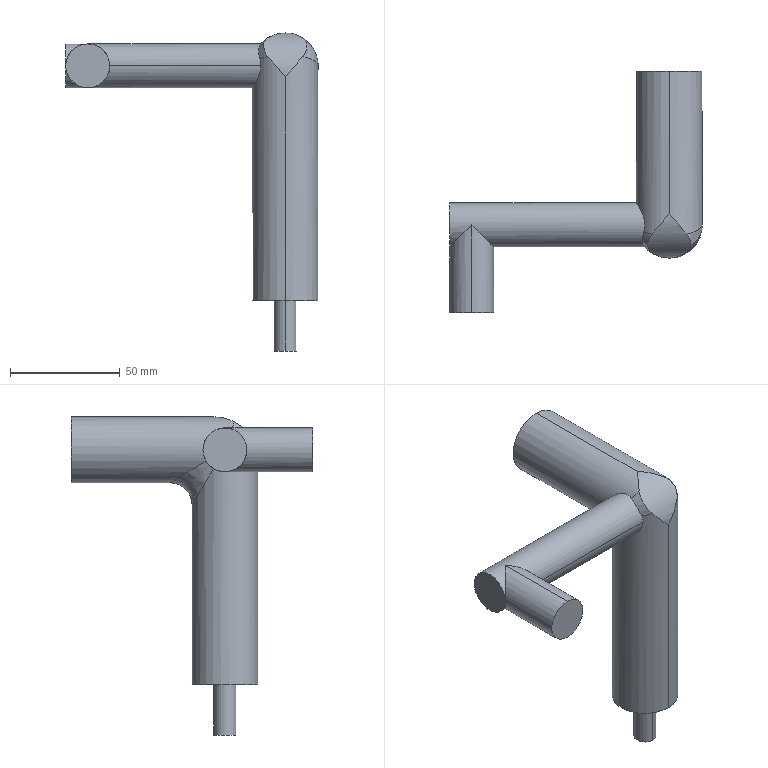Part | SolidWorks | features BaseBody 1 | 1 solid | 19 faces | box 115 x 110 x 145 mm | volume 163040 mm3 | cylinder 11 | plane 5 | spline 3 | commonest cylinder face diameters 20 x4 30 x4 10 x2 40 x1
STEP:
#1=CARTESIAN_POINT('',(268.959,17.138,-340.));
#2=VERTEX_POINT('',#1);
#3=CARTESIAN_POINT('',(268.959,17.138,-360.));
#4=VERTEX_POINT('',#3);
#5=CARTESIAN_POINT('',(268.959,17.138,-350.));
#6=DIRECTION('',(0.,-1.,0.));
#7=DIRECTION('',(0.,0.,1.));
#8=AXIS2_PLACEMENT_3D('',#5,#6,#7);
#9=CIRCLE('',#8,10.);
#10=EDGE_CURVE('',#2,#4,#9,.T.);
#11=ORIENTED_EDGE('',*,*,#10,.F.);
#12=CARTESIAN_POINT('',(268.959,57.138,-340.));
#13=VERTEX_POINT('',#12);
#14=CARTESIAN_POINT('',(268.959,17.138,-340.));
#15=DIRECTION('',(0.,1.,0.));
#16=VECTOR('',#15,1000.);
#17=LINE('',#14,#16);
#18=EDGE_CURVE('',#2,#13,#17,.T.);
#19=ORIENTED_EDGE('',*,*,#18,.T.);
#20=CARTESIAN_POINT('',(258.959,47.138,-350.));
#21=VERTEX_POINT('',#20);
#22=CARTESIAN_POINT('',(268.959,57.138,-340.));
#23=CARTESIAN_POINT('',(263.101,51.28,-340.));
#24=CARTESIAN_POINT('',(258.959,47.138,-344.142));
#25=CARTESIAN_POINT('',(258.959,47.138,-350.));
#26=(BOUNDED_CURVE()B_SPLINE_CURVE(3,(#22,#23,#24,#25),.UNSPECIFIED.,.F.,.T.)B_SPLINE_CURVE_WITH_KNOTS((4,4),(1.571,3.142),.UNSPECIFIED.)CURVE()GEOMETRIC_REPRESENTATION_ITEM()RATIONAL_B_SPLINE_CURVE((1.,0.8047,0.8047,1.))REPRESENTATION_ITEM(''));
#27=EDGE_CURVE('',#13,#21,#26,.T.);
#28=ORIENTED_EDGE('',*,*,#27,.T.);
#29=CARTESIAN_POINT('',(268.959,57.138,-360.));
#30=VERTEX_POINT('',#29);
#31=CARTESIAN_POINT('',(258.959,47.138,-350.));
#32=CARTESIAN_POINT('',(258.959,47.138,-355.858));
#33=CARTESIAN_POINT('',(263.101,51.28,-360.));
#34=CARTESIAN_POINT('',(268.959,57.138,-360.));
#35=(BOUNDED_CURVE()B_SPLINE_CURVE(3,(#31,#32,#33,#34),.UNSPECIFIED.,.F.,.F.)B_SPLINE_CURVE_WITH_KNOTS((4,4),(3.142,4.712),.UNSPECIFIED.)CURVE()GEOMETRIC_REPRESENTATION_ITEM()RATIONAL_B_SPLINE_CURVE((1.,0.8047,0.8047,1.))REPRESENTATION_ITEM(''));
#36=EDGE_CURVE('',#21,#30,#35,.T.);
#37=ORIENTED_EDGE('',*,*,#36,.T.);
#38=CARTESIAN_POINT('',(268.959,17.138,-360.));
#39=DIRECTION('',(0.,1.,0.));
#40=VECTOR('',#39,1000.);
#41=LINE('',#38,#40);
#42=EDGE_CURVE('',#4,#30,#41,.T.);
#43=ORIENTED_EDGE('',*,*,#42,.F.);
#44=EDGE_LOOP('',(#11,#19,#28,#37,#43));
#45=FACE_OUTER_BOUND('',#44,.T.);
#46=CARTESIAN_POINT('',(268.959,17.138,-350.));
#47=DIRECTION('',(0.,1.,0.));
#48=DIRECTION('',(0.,0.,-1.));
#49=AXIS2_PLACEMENT_3D('',#46,#47,#48);
#50=CYLINDRICAL_SURFACE('',#49,10.);
#51=ADVANCED_FACE('',(#45),#50,.T.);
#52=CARTESIAN_POINT('',(358.959,52.138,-480.));
#53=VERTEX_POINT('',#52);
#54=CARTESIAN_POINT('',(358.959,62.138,-480.));
#55=VERTEX_POINT('',#54);
#56=CARTESIAN_POINT('',(358.959,57.138,-480.));
#57=DIRECTION('',(0.,0.,-1.));
#58=DIRECTION('',(0.,-1.,0.));
#59=AXIS2_PLACEMENT_3D('',#56,#57,#58);
#60=CIRCLE('',#59,5.);
#61=EDGE_CURVE('',#53,#55,#60,.T.);
#62=ORIENTED_EDGE('',*,*,#61,.F.);
#63=CARTESIAN_POINT('',(358.959,52.138,-457.));
#64=VERTEX_POINT('',#63);
#65=CARTESIAN_POINT('',(358.959,52.138,-480.));
#66=DIRECTION('',(0.,0.,1.));
#67=VECTOR('',#66,1000.);
#68=LINE('',#65,#67);
#69=EDGE_CURVE('',#53,#64,#68,.T.);
#70=ORIENTED_EDGE('',*,*,#69,.T.);
#71=CARTESIAN_POINT('',(358.959,62.138,-457.));
#72=VERTEX_POINT('',#71);
#73=CARTESIAN_POINT('',(358.959,57.138,-457.));
#74=DIRECTION('',(0.,0.,-1.));
#75=DIRECTION('',(0.,1.,0.));
#76=AXIS2_PLACEMENT_3D('',#73,#74,#75);
#77=CIRCLE('',#76,5.);
#78=EDGE_CURVE('',#64,#72,#77,.T.);
#79=ORIENTED_EDGE('',*,*,#78,.T.);
#80=CARTESIAN_POINT('',(358.959,62.138,-480.));
#81=DIRECTION('',(0.,0.,1.));
#82=VECTOR('',#81,1000.);
#83=LINE('',#80,#82);
#84=EDGE_CURVE('',#55,#72,#83,.T.);
#85=ORIENTED_EDGE('',*,*,#84,.F.);
#86=EDGE_LOOP('',(#62,#70,#79,#85));
#87=FACE_OUTER_BOUND('',#86,.T.);
#88=CARTESIAN_POINT('',(358.959,57.138,-480.));
#89=DIRECTION('',(0.,0.,1.));
#90=DIRECTION('',(0.,1.,0.));
#91=AXIS2_PLACEMENT_3D('',#88,#89,#90);
#92=CYLINDRICAL_SURFACE('',#91,5.);
#93=ADVANCED_FACE('',(#87),#92,.T.);
#94=CARTESIAN_POINT('',(344.869,62.283,-358.575));
#95=VERTEX_POINT('',#94);
#96=CARTESIAN_POINT('',(358.959,72.138,-375.));
#97=VERTEX_POINT('',#96);
#98=CARTESIAN_POINT('',(344.869,62.283,-358.575));
#99=CARTESIAN_POINT('',(347.104,68.404,-368.776));
#100=CARTESIAN_POINT('',(352.443,72.138,-375.));
#101=CARTESIAN_POINT('',(358.959,72.138,-375.));
#102=(BOUNDED_CURVE()B_SPLINE_CURVE(3,(#98,#99,#100,#101),.UNSPECIFIED.,.F.,.T.)B_SPLINE_CURVE_WITH_KNOTS((4,4),(5.062,6.283),.UNSPECIFIED.)CURVE()GEOMETRIC_REPRESENTATION_ITEM()RATIONAL_B_SPLINE_CURVE((1.,0.8796,0.8796,1.))REPRESENTATION_ITEM(''));
#103=EDGE_CURVE('',#95,#97,#102,.T.);
#104=ORIENTED_EDGE('',*,*,#103,.T.);
#105=CARTESIAN_POINT('',(358.959,72.138,-457.));
#106=VERTEX_POINT('',#105);
#107=CARTESIAN_POINT('',(358.959,72.138,-307.574));
#108=DIRECTION('',(0.,0.,-1.));
#109=VECTOR('',#108,1000.);
#110=LINE('',#107,#109);
#111=EDGE_CURVE('',#97,#106,#110,.T.);
#112=ORIENTED_EDGE('',*,*,#111,.T.);
#113=CARTESIAN_POINT('',(358.959,42.138,-457.));
#114=VERTEX_POINT('',#113);
#115=CARTESIAN_POINT('',(358.959,57.138,-457.));
#116=DIRECTION('',(0.,0.,1.));
#117=DIRECTION('',(0.,1.,0.));
#118=AXIS2_PLACEMENT_3D('',#115,#116,#117);
#119=CIRCLE('',#118,15.);
#120=EDGE_CURVE('',#106,#114,#119,.T.);
#121=ORIENTED_EDGE('',*,*,#120,.T.);
#122=CARTESIAN_POINT('',(358.959,42.138,-355.));
#123=VERTEX_POINT('',#122);
#124=CARTESIAN_POINT('',(358.959,42.138,-307.574));
#125=DIRECTION('',(0.,0.,-1.));
#126=VECTOR('',#125,1000.);
#127=LINE('',#124,#126);
#128=EDGE_CURVE('',#123,#114,#127,.T.);
#129=ORIENTED_EDGE('',*,*,#128,.F.);
#130=CARTESIAN_POINT('',(351.033,44.403,-345.755));
#131=VERTEX_POINT('',#130);
#132=CARTESIAN_POINT('',(358.959,42.138,-355.));
#133=CARTESIAN_POINT('',(358.789,42.138,-354.804));
#134=CARTESIAN_POINT('',(358.618,42.141,-354.606));
#135=CARTESIAN_POINT('',(358.277,42.153,-354.212));
#136=CARTESIAN_POINT('',(358.106,42.162,-354.015));
#137=CARTESIAN_POINT('',(357.596,42.197,-353.426));
#138=CARTESIAN_POINT('',(357.257,42.231,-353.034));
#139=CARTESIAN_POINT('',(356.242,42.371,-351.86));
#140=CARTESIAN_POINT('',(355.569,42.51,-351.08));
#141=CARTESIAN_POINT('',(354.567,42.792,-349.915));
#142=CARTESIAN_POINT('',(354.234,42.898,-349.526));
#143=CARTESIAN_POINT('',(353.574,43.134,-348.756));
#144=CARTESIAN_POINT('',(353.248,43.264,-348.374));
#145=CARTESIAN_POINT('',(352.28,43.689,-347.236));
#146=CARTESIAN_POINT('',(351.649,44.02,-346.49));
#147=CARTESIAN_POINT('',(351.033,44.403,-345.755));
#148=B_SPLINE_CURVE_WITH_KNOTS('',3,(#132,#133,#134,#135,#136,#137,#138,#139,#140,#141,#142,#143,#144,#145,#146,#147),.UNSPECIFIED.,.F.,.F.,(4,2,2,2,2,2,2,4),(-0.00002828,0.0007507,0.00153,0.003088,0.006204,0.007762,0.00932,0.01244),.UNSPECIFIED.);
#149=EDGE_CURVE('',#123,#131,#148,.T.);
#150=ORIENTED_EDGE('',*,*,#149,.T.);
#151=CARTESIAN_POINT('',(347.34,47.652,-346.838));
#152=VERTEX_POINT('',#151);
#153=CARTESIAN_POINT('',(351.033,44.403,-345.755));
#154=CARTESIAN_POINT('',(349.629,45.277,-346.046));
#155=CARTESIAN_POINT('',(348.386,46.37,-346.411));
#156=CARTESIAN_POINT('',(347.34,47.652,-346.838));
#157=(BOUNDED_CURVE()B_SPLINE_CURVE(3,(#153,#154,#155,#156),.UNSPECIFIED.,.F.,.F.)B_SPLINE_CURVE_WITH_KNOTS((4,4),(3.698,4.028),.UNSPECIFIED.)CURVE()GEOMETRIC_REPRESENTATION_ITEM()RATIONAL_B_SPLINE_CURVE((1.,0.991,0.991,1.))REPRESENTATION_ITEM(''));
#158=EDGE_CURVE('',#131,#152,#157,.T.);
#159=ORIENTED_EDGE('',*,*,#158,.T.);
#160=CARTESIAN_POINT('',(347.779,47.138,-350.));
#161=VERTEX_POINT('',#160);
#162=CARTESIAN_POINT('',(347.779,47.138,-350.));
#163=CARTESIAN_POINT('',(347.779,47.138,-349.458));
#164=CARTESIAN_POINT('',(347.739,47.182,-348.921));
#165=CARTESIAN_POINT('',(347.626,47.312,-348.125));
#166=CARTESIAN_POINT('',(347.579,47.367,-347.859));
#167=CARTESIAN_POINT('',(347.47,47.495,-347.341));
#168=CARTESIAN_POINT('',(347.408,47.569,-347.087));
#169=CARTESIAN_POINT('',(347.34,47.652,-346.838));
#170=B_SPLINE_CURVE_WITH_KNOTS('',3,(#162,#163,#164,#165,#166,#167,#168,#169),.UNSPECIFIED.,.F.,.F.,(4,2,2,4),(0.0323,0.03391,0.03472,0.03552),.UNSPECIFIED.);
#171=EDGE_CURVE('',#161,#152,#170,.T.);
#172=ORIENTED_EDGE('',*,*,#171,.F.);
#173=CARTESIAN_POINT('',(344.869,62.283,-358.575));
#174=CARTESIAN_POINT('',(344.735,61.916,-358.796));
#175=CARTESIAN_POINT('',(344.611,61.532,-358.994));
#176=CARTESIAN_POINT('',(344.445,60.931,-359.256));
#177=CARTESIAN_POINT('',(344.393,60.726,-359.337));
#178=CARTESIAN_POINT('',(344.296,60.307,-359.487));
#179=CARTESIAN_POINT('',(344.251,60.092,-359.556));
#180=CARTESIAN_POINT('',(344.052,59.017,-359.862));
#181=CARTESIAN_POINT('',(343.964,58.133,-359.992));
#182=CARTESIAN_POINT('',(343.958,56.994,-360.002));
#183=CARTESIAN_POINT('',(343.962,56.764,-359.996));
#184=CARTESIAN_POINT('',(343.98,56.31,-359.968));
#185=CARTESIAN_POINT('',(343.995,56.085,-359.947));
#186=CARTESIAN_POINT('',(344.052,55.414,-359.861));
#187=CARTESIAN_POINT('',(344.11,54.974,-359.773));
#188=CARTESIAN_POINT('',(344.262,54.108,-359.54));
#189=CARTESIAN_POINT('',(344.357,53.682,-359.394));
#190=CARTESIAN_POINT('',(344.573,52.87,-359.054));
#191=CARTESIAN_POINT('',(344.695,52.48,-358.859));
#192=CARTESIAN_POINT('',(344.963,51.729,-358.422));
#193=CARTESIAN_POINT('',(345.109,51.368,-358.178));
#194=CARTESIAN_POINT('',(345.411,50.69,-357.655));
#195=CARTESIAN_POINT('',(345.568,50.371,-357.375));
#196=CARTESIAN_POINT('',(345.888,49.772,-356.776));
#197=CARTESIAN_POINT('',(346.052,49.489,-356.455));
#198=CARTESIAN_POINT('',(346.376,48.968,-355.781));
#199=CARTESIAN_POINT('',(346.534,48.73,-355.43));
#200=CARTESIAN_POINT('',(346.837,48.3,-354.698));
#201=CARTESIAN_POINT('',(346.98,48.108,-354.317));
#202=CARTESIAN_POINT('',(347.244,47.768,-353.519));
#203=CARTESIAN_POINT('',(347.365,47.62,-353.1));
#204=CARTESIAN_POINT('',(347.563,47.383,-352.244));
#205=CARTESIAN_POINT('',(347.642,47.293,-351.808));
#206=CARTESIAN_POINT('',(347.75,47.17,-350.915));
#207=CARTESIAN_POINT('',(347.779,47.138,-350.454));
#208=CARTESIAN_POINT('',(347.779,47.138,-350.));
#209=B_SPLINE_CURVE_WITH_KNOTS('',3,(#173,#174,#175,#176,#177,#178,#179,#180,#181,#182,#183,#184,#185,#186,#187,#188,#189,#190,#191,#192,#193,#194,#195,#196,#197,#198,#199,#200,#201,#202,#203,#204,#205,#206,#207,#208),.UNSPECIFIED.,.F.,.F.,(4,2,2,2,2,2,2,2,2,2,2,2,2,2,2,2,2,4),(0.01069,0.01204,0.01272,0.01339,0.01609,0.01677,0.01744,0.01879,0.02014,0.02149,0.02285,0.0242,0.02555,0.0269,0.02825,0.0296,0.03095,0.0323),.UNSPECIFIED.);
#210=EDGE_CURVE('',#95,#161,#209,.T.);
#211=ORIENTED_EDGE('',*,*,#210,.F.);
#212=EDGE_LOOP('',(#104,#112,#121,#129,#150,#159,#172,#211));
#213=FACE_OUTER_BOUND('',#212,.T.);
#214=CARTESIAN_POINT('',(358.959,57.138,-307.574));
#215=DIRECTION('',(0.,0.,-1.));
#216=DIRECTION('',(0.,-1.,0.));
#217=AXIS2_PLACEMENT_3D('',#214,#215,#216);
#218=CYLINDRICAL_SURFACE('',#217,15.);
#219=ADVANCED_FACE('',(#213),#218,.T.);
#220=CARTESIAN_POINT('',(358.959,62.138,-335.));
#221=VERTEX_POINT('',#220);
#222=CARTESIAN_POINT('',(351.033,52.893,-337.265));
#223=VERTEX_POINT('',#222);
#224=CARTESIAN_POINT('',(358.959,62.138,-335.));
#225=CARTESIAN_POINT('',(358.789,61.942,-335.));
#226=CARTESIAN_POINT('',(358.618,61.744,-335.003));
#227=CARTESIAN_POINT('',(358.277,61.35,-335.015));
#228=CARTESIAN_POINT('',(358.106,61.154,-335.023));
#229=CARTESIAN_POINT('',(357.596,60.564,-335.058));
#230=CARTESIAN_POINT('',(357.257,60.172,-335.093));
#231=CARTESIAN_POINT('',(356.242,58.998,-335.232));
#232=CARTESIAN_POINT('',(355.569,58.219,-335.372));
#233=CARTESIAN_POINT('',(354.567,57.053,-335.653));
#234=CARTESIAN_POINT('',(354.234,56.664,-335.76));
#235=CARTESIAN_POINT('',(353.574,55.894,-335.995));
#236=CARTESIAN_POINT('',(353.248,55.512,-336.125));
#237=CARTESIAN_POINT('',(352.28,54.375,-336.551));
#238=CARTESIAN_POINT('',(351.649,53.628,-336.882));
#239=CARTESIAN_POINT('',(351.033,52.893,-337.265));
#240=B_SPLINE_CURVE_WITH_KNOTS('',3,(#224,#225,#226,#227,#228,#229,#230,#231,#232,#233,#234,#235,#236,#237,#238,#239),.UNSPECIFIED.,.F.,.F.,(4,2,2,2,2,2,2,4),(-0.00002828,0.0007507,0.00153,0.003088,0.006204,0.007762,0.00932,0.01244),.UNSPECIFIED.);
#241=EDGE_CURVE('',#221,#223,#240,.T.);
#242=ORIENTED_EDGE('',*,*,#241,.F.);
#243=CARTESIAN_POINT('',(358.959,127.138,-335.));
#244=VERTEX_POINT('',#243);
#245=CARTESIAN_POINT('',(358.959,57.138,-335.));
#246=DIRECTION('',(0.,1.,0.));
#247=VECTOR('',#246,1000.);
#248=LINE('',#245,#247);
#249=EDGE_CURVE('',#221,#244,#248,.T.);
#250=ORIENTED_EDGE('',*,*,#249,.T.);
#251=CARTESIAN_POINT('',(358.959,127.138,-365.));
#252=VERTEX_POINT('',#251);
#253=CARTESIAN_POINT('',(358.959,127.138,-350.));
#254=DIRECTION('',(0.,-1.,0.));
#255=DIRECTION('',(0.,0.,-1.));
#256=AXIS2_PLACEMENT_3D('',#253,#254,#255);
#257=CIRCLE('',#256,15.);
#258=EDGE_CURVE('',#244,#252,#257,.T.);
#259=ORIENTED_EDGE('',*,*,#258,.T.);
#260=CARTESIAN_POINT('',(358.959,82.138,-365.));
#261=VERTEX_POINT('',#260);
#262=CARTESIAN_POINT('',(358.959,57.138,-365.));
#263=DIRECTION('',(0.,1.,0.));
#264=VECTOR('',#263,1000.);
#265=LINE('',#262,#264);
#266=EDGE_CURVE('',#261,#252,#265,.T.);
#267=ORIENTED_EDGE('',*,*,#266,.F.);
#268=CARTESIAN_POINT('',(344.869,65.713,-355.145));
#269=VERTEX_POINT('',#268);
#270=CARTESIAN_POINT('',(358.959,82.138,-365.));
#271=CARTESIAN_POINT('',(352.443,82.138,-365.));
#272=CARTESIAN_POINT('',(347.104,75.914,-361.265));
#273=CARTESIAN_POINT('',(344.869,65.713,-355.145));
#274=(BOUNDED_CURVE()B_SPLINE_CURVE(3,(#270,#271,#272,#273),.UNSPECIFIED.,.F.,.F.)B_SPLINE_CURVE_WITH_KNOTS((4,4),(0.,1.221),.UNSPECIFIED.)CURVE()GEOMETRIC_REPRESENTATION_ITEM()RATIONAL_B_SPLINE_CURVE((1.,0.8796,0.8796,1.))REPRESENTATION_ITEM(''));
#275=EDGE_CURVE('',#261,#269,#274,.T.);
#276=ORIENTED_EDGE('',*,*,#275,.T.);
#277=CARTESIAN_POINT('',(343.959,67.138,-350.));
#278=VERTEX_POINT('',#277);
#279=CARTESIAN_POINT('',(344.869,65.713,-355.145));
#280=CARTESIAN_POINT('',(344.733,65.937,-354.772));
#281=CARTESIAN_POINT('',(344.608,66.137,-354.383));
#282=CARTESIAN_POINT('',(344.44,66.401,-353.775));
#283=CARTESIAN_POINT('',(344.388,66.483,-353.567));
#284=CARTESIAN_POINT('',(344.291,66.634,-353.144));
#285=CARTESIAN_POINT('',(344.246,66.703,-352.926));
#286=CARTESIAN_POINT('',(344.125,66.888,-352.269));
#287=CARTESIAN_POINT('',(344.064,66.981,-351.824));
#288=CARTESIAN_POINT('',(343.981,67.106,-350.922));
#289=CARTESIAN_POINT('',(343.959,67.138,-350.463));
#290=CARTESIAN_POINT('',(343.959,67.138,-350.));
#291=B_SPLINE_CURVE_WITH_KNOTS('',3,(#279,#280,#281,#282,#283,#284,#285,#286,#287,#288,#289,#290),.UNSPECIFIED.,.F.,.F.,(4,2,2,2,2,4),(0.05913,0.06049,0.06118,0.06186,0.06323,0.0646),.UNSPECIFIED.);
#292=EDGE_CURVE('',#269,#278,#291,.T.);
#293=ORIENTED_EDGE('',*,*,#292,.T.);
#294=CARTESIAN_POINT('',(347.34,53.976,-340.513));
#295=VERTEX_POINT('',#294);
#296=CARTESIAN_POINT('',(343.959,67.138,-350.));
#297=CARTESIAN_POINT('',(343.959,67.138,-349.179));
#298=CARTESIAN_POINT('',(344.026,67.039,-348.379));
#299=CARTESIAN_POINT('',(344.216,66.749,-347.209));
#300=CARTESIAN_POINT('',(344.295,66.628,-346.822));
#301=CARTESIAN_POINT('',(344.475,66.347,-346.081));
#302=CARTESIAN_POINT('',(344.577,66.186,-345.723));
#303=CARTESIAN_POINT('',(344.801,65.826,-345.032));
#304=CARTESIAN_POINT('',(344.923,65.626,-344.697));
#305=CARTESIAN_POINT('',(345.183,65.189,-344.055));
#306=CARTESIAN_POINT('',(345.319,64.955,-343.751));
#307=CARTESIAN_POINT('',(345.598,64.457,-343.175));
#308=CARTESIAN_POINT('',(345.741,64.193,-342.903));
#309=CARTESIAN_POINT('',(346.031,63.634,-342.388));
#310=CARTESIAN_POINT('',(346.178,63.338,-342.144));
#311=CARTESIAN_POINT('',(346.608,62.414,-341.471));
#312=CARTESIAN_POINT('',(346.882,61.754,-341.095));
#313=CARTESIAN_POINT('',(347.235,60.683,-340.641));
#314=CARTESIAN_POINT('',(347.344,60.308,-340.507));
#315=CARTESIAN_POINT('',(347.529,59.544,-340.286));
#316=CARTESIAN_POINT('',(347.605,59.156,-340.197));
#317=CARTESIAN_POINT('',(347.719,58.363,-340.067));
#318=CARTESIAN_POINT('',(347.756,57.957,-340.025));
#319=CARTESIAN_POINT('',(347.786,57.138,-339.992));
#320=CARTESIAN_POINT('',(347.779,56.732,-340.));
#321=CARTESIAN_POINT('',(347.721,55.927,-340.065));
#322=CARTESIAN_POINT('',(347.67,55.528,-340.122));
#323=CARTESIAN_POINT('',(347.53,54.736,-340.284));
#324=CARTESIAN_POINT('',(347.442,54.35,-340.389));
#325=CARTESIAN_POINT('',(347.34,53.976,-340.513));
#326=B_SPLINE_CURVE_WITH_KNOTS('',3,(#296,#297,#298,#299,#300,#301,#302,#303,#304,#305,#306,#307,#308,#309,#310,#311,#312,#313,#314,#315,#316,#317,#318,#319,#320,#321,#322,#323,#324,#325),.UNSPECIFIED.,.F.,.F.,(4,2,2,2,2,2,2,2,2,2,2,2,2,2,4),(0.,0.002425,0.003638,0.00485,0.006063,0.007275,0.008488,0.009701,0.01213,0.01334,0.01455,0.01576,0.01698,0.01819,0.0194),.UNSPECIFIED.);
#327=EDGE_CURVE('',#278,#295,#326,.T.);
#328=ORIENTED_EDGE('',*,*,#327,.T.);
#329=CARTESIAN_POINT('',(347.34,53.976,-340.513));
#330=CARTESIAN_POINT('',(348.386,53.549,-339.232));
#331=CARTESIAN_POINT('',(349.629,53.185,-338.139));
#332=CARTESIAN_POINT('',(351.033,52.893,-337.265));
#333=(BOUNDED_CURVE()B_SPLINE_CURVE(3,(#329,#330,#331,#332),.UNSPECIFIED.,.F.,.T.)B_SPLINE_CURVE_WITH_KNOTS((4,4),(2.256,2.585),.UNSPECIFIED.)CURVE()GEOMETRIC_REPRESENTATION_ITEM()RATIONAL_B_SPLINE_CURVE((1.,0.991,0.991,1.))REPRESENTATION_ITEM(''));
#334=EDGE_CURVE('',#295,#223,#333,.T.);
#335=ORIENTED_EDGE('',*,*,#334,.T.);
#336=EDGE_LOOP('',(#242,#250,#259,#267,#276,#293,#328,#335));
#337=FACE_OUTER_BOUND('',#336,.T.);
#338=CARTESIAN_POINT('',(358.959,57.138,-350.));
#339=DIRECTION('',(0.,1.,0.));
#340=DIRECTION('',(0.,0.,-1.));
#341=AXIS2_PLACEMENT_3D('',#338,#339,#340);
#342=CYLINDRICAL_SURFACE('',#341,15.);
#343=ADVANCED_FACE('',(#337),#342,.T.);
#344=CARTESIAN_POINT('',(278.959,47.138,-350.));
#345=VERTEX_POINT('',#344);
#346=CARTESIAN_POINT('',(278.959,47.138,-350.));
#347=CARTESIAN_POINT('',(278.959,47.138,-344.142));
#348=CARTESIAN_POINT('',(274.817,51.28,-340.));
#349=CARTESIAN_POINT('',(268.959,57.138,-340.));
#350=(BOUNDED_CURVE()B_SPLINE_CURVE(3,(#346,#347,#348,#349),.UNSPECIFIED.,.F.,.T.)B_SPLINE_CURVE_WITH_KNOTS((4,4),(0.,1.571),.UNSPECIFIED.)CURVE()GEOMETRIC_REPRESENTATION_ITEM()RATIONAL_B_SPLINE_CURVE((1.,0.8047,0.8047,1.))REPRESENTATION_ITEM(''));
#351=EDGE_CURVE('',#345,#13,#350,.T.);
#352=ORIENTED_EDGE('',*,*,#351,.F.);
#353=CARTESIAN_POINT('',(258.959,47.138,-350.));
#354=DIRECTION('',(1.,0.,0.));
#355=VECTOR('',#354,1000.);
#356=LINE('',#353,#355);
#357=EDGE_CURVE('',#345,#161,#356,.T.);
#358=ORIENTED_EDGE('',*,*,#357,.T.);
#359=ORIENTED_EDGE('',*,*,#171,.T.);
#360=CARTESIAN_POINT('',(347.34,47.652,-346.838));
#361=CARTESIAN_POINT('',(347.143,47.893,-346.114));
#362=CARTESIAN_POINT('',(346.996,48.215,-345.421));
#363=CARTESIAN_POINT('',(346.845,48.823,-344.432));
#364=CARTESIAN_POINT('',(346.807,49.049,-344.109));
#365=CARTESIAN_POINT('',(346.756,49.532,-343.496));
#366=CARTESIAN_POINT('',(346.744,49.791,-343.206));
#367=CARTESIAN_POINT('',(346.743,50.34,-342.656));
#368=CARTESIAN_POINT('',(346.756,50.631,-342.397));
#369=CARTESIAN_POINT('',(346.806,51.246,-341.911));
#370=CARTESIAN_POINT('',(346.845,51.567,-341.687));
#371=CARTESIAN_POINT('',(346.945,52.225,-341.282));
#372=CARTESIAN_POINT('',(347.007,52.563,-341.1));
#373=CARTESIAN_POINT('',(347.155,53.257,-340.776));
#374=CARTESIAN_POINT('',(347.242,53.614,-340.634));
#375=CARTESIAN_POINT('',(347.34,53.976,-340.513));
#376=B_SPLINE_CURVE_WITH_KNOTS('',3,(#360,#361,#362,#363,#364,#365,#366,#367,#368,#369,#370,#371,#372,#373,#374,#375),.UNSPECIFIED.,.F.,.F.,(4,2,2,2,2,2,2,4),(0.,0.002332,0.003498,0.004664,0.00583,0.006996,0.008162,0.009328),.UNSPECIFIED.);
#377=EDGE_CURVE('',#152,#295,#376,.T.);
#378=ORIENTED_EDGE('',*,*,#377,.T.);
#379=ORIENTED_EDGE('',*,*,#327,.F.);
#380=CARTESIAN_POINT('',(258.959,67.138,-350.));
#381=VERTEX_POINT('',#380);
#382=CARTESIAN_POINT('',(258.959,67.138,-350.));
#383=DIRECTION('',(1.,0.,0.));
#384=VECTOR('',#383,1000.);
#385=LINE('',#382,#384);
#386=EDGE_CURVE('',#381,#278,#385,.T.);
#387=ORIENTED_EDGE('',*,*,#386,.F.);
#388=CARTESIAN_POINT('',(258.959,57.138,-350.));
#389=DIRECTION('',(-1.,0.,0.));
#390=DIRECTION('',(0.,-1.,0.));
#391=AXIS2_PLACEMENT_3D('',#388,#389,#390);
#392=CIRCLE('',#391,10.);
#393=EDGE_CURVE('',#21,#381,#392,.T.);
#394=ORIENTED_EDGE('',*,*,#393,.F.);
#395=ORIENTED_EDGE('',*,*,#27,.F.);
#396=EDGE_LOOP('',(#352,#358,#359,#378,#379,#387,#394,#395));
#397=FACE_OUTER_BOUND('',#396,.T.);
#398=CARTESIAN_POINT('',(258.959,57.138,-350.));
#399=DIRECTION('',(1.,0.,0.));
#400=DIRECTION('',(0.,1.,0.));
#401=AXIS2_PLACEMENT_3D('',#398,#399,#400);
#402=CYLINDRICAL_SURFACE('',#401,10.);
#403=ADVANCED_FACE('',(#397),#402,.T.);
#404=ORIENTED_EDGE('',*,*,#357,.F.);
#405=CARTESIAN_POINT('',(268.959,57.138,-360.));
#406=CARTESIAN_POINT('',(274.817,51.28,-360.));
#407=CARTESIAN_POINT('',(278.959,47.138,-355.858));
#408=CARTESIAN_POINT('',(278.959,47.138,-350.));
#409=(BOUNDED_CURVE()B_SPLINE_CURVE(3,(#405,#406,#407,#408),.UNSPECIFIED.,.F.,.T.)B_SPLINE_CURVE_WITH_KNOTS((4,4),(4.712,6.283),.UNSPECIFIED.)CURVE()GEOMETRIC_REPRESENTATION_ITEM()RATIONAL_B_SPLINE_CURVE((1.,0.8047,0.8047,1.))REPRESENTATION_ITEM(''));
#410=EDGE_CURVE('',#30,#345,#409,.T.);
#411=ORIENTED_EDGE('',*,*,#410,.F.);
#412=ORIENTED_EDGE('',*,*,#36,.F.);
#413=CARTESIAN_POINT('',(258.959,57.138,-350.));
#414=DIRECTION('',(-1.,0.,0.));
#415=DIRECTION('',(0.,-1.,0.));
#416=AXIS2_PLACEMENT_3D('',#413,#414,#415);
#417=CIRCLE('',#416,10.);
#418=EDGE_CURVE('',#381,#21,#417,.T.);
#419=ORIENTED_EDGE('',*,*,#418,.F.);
#420=ORIENTED_EDGE('',*,*,#386,.T.);
#421=ORIENTED_EDGE('',*,*,#292,.F.);
#422=CARTESIAN_POINT('',(344.869,65.713,-355.145));
#423=CARTESIAN_POINT('',(344.994,65.508,-355.487));
#424=CARTESIAN_POINT('',(345.091,65.281,-355.819));
#425=CARTESIAN_POINT('',(345.189,64.905,-356.302));
#426=CARTESIAN_POINT('',(345.214,64.775,-356.46));
#427=CARTESIAN_POINT('',(345.248,64.5,-356.771));
#428=CARTESIAN_POINT('',(345.257,64.357,-356.924));
#429=CARTESIAN_POINT('',(345.257,63.916,-357.365));
#430=CARTESIAN_POINT('',(345.223,63.608,-357.636));
#431=CARTESIAN_POINT('',(345.092,62.963,-358.139));
#432=CARTESIAN_POINT('',(344.994,62.626,-358.369));
#433=CARTESIAN_POINT('',(344.869,62.283,-358.575));
#434=B_SPLINE_CURVE_WITH_KNOTS('',3,(#422,#423,#424,#425,#426,#427,#428,#429,#430,#431,#432,#433),.UNSPECIFIED.,.F.,.F.,(4,2,2,2,2,4),(0.,0.001238,0.001857,0.002476,0.003714,0.004952),.UNSPECIFIED.);
#435=EDGE_CURVE('',#269,#95,#434,.T.);
#436=ORIENTED_EDGE('',*,*,#435,.T.);
#437=ORIENTED_EDGE('',*,*,#210,.T.);
#438=EDGE_LOOP('',(#404,#411,#412,#419,#420,#421,#436,#437));
#439=FACE_OUTER_BOUND('',#438,.T.);
#440=CARTESIAN_POINT('',(258.959,57.138,-350.));
#441=DIRECTION('',(1.,0.,0.));
#442=DIRECTION('',(0.,1.,0.));
#443=AXIS2_PLACEMENT_3D('',#440,#441,#442);
#444=CYLINDRICAL_SURFACE('',#443,10.);
#445=ADVANCED_FACE('',(#439),#444,.T.);
#446=ORIENTED_EDGE('',*,*,#249,.F.);
#447=CARTESIAN_POINT('',(366.885,52.893,-337.265));
#448=VERTEX_POINT('',#447);
#449=CARTESIAN_POINT('',(366.885,52.893,-337.265));
#450=CARTESIAN_POINT('',(366.27,53.628,-336.882));
#451=CARTESIAN_POINT('',(365.638,54.375,-336.551));
#452=CARTESIAN_POINT('',(364.67,55.512,-336.125));
#453=CARTESIAN_POINT('',(364.344,55.894,-335.995));
#454=CARTESIAN_POINT('',(363.685,56.664,-335.759));
#455=CARTESIAN_POINT('',(363.351,57.053,-335.653));
#456=CARTESIAN_POINT('',(362.349,58.219,-335.372));
#457=CARTESIAN_POINT('',(361.676,58.998,-335.232));
#458=CARTESIAN_POINT('',(360.661,60.172,-335.093));
#459=CARTESIAN_POINT('',(360.322,60.564,-335.058));
#460=CARTESIAN_POINT('',(359.812,61.154,-335.023));
#461=CARTESIAN_POINT('',(359.642,61.35,-335.015));
#462=CARTESIAN_POINT('',(359.301,61.744,-335.003));
#463=CARTESIAN_POINT('',(359.129,61.942,-335.));
#464=CARTESIAN_POINT('',(358.959,62.138,-335.));
#465=B_SPLINE_CURVE_WITH_KNOTS('',3,(#449,#450,#451,#452,#453,#454,#455,#456,#457,#458,#459,#460,#461,#462,#463,#464),.UNSPECIFIED.,.F.,.F.,(4,2,2,2,2,2,2,4),(0.02356,0.02667,0.02823,0.02978,0.03289,0.03445,0.03523,0.036),.UNSPECIFIED.);
#466=EDGE_CURVE('',#448,#221,#465,.T.);
#467=ORIENTED_EDGE('',*,*,#466,.F.);
#468=CARTESIAN_POINT('',(373.959,57.138,-350.));
#469=VERTEX_POINT('',#468);
#470=CARTESIAN_POINT('',(366.885,52.893,-337.265));
#471=CARTESIAN_POINT('',(371.385,53.827,-340.066));
#472=CARTESIAN_POINT('',(373.959,55.371,-344.699));
#473=CARTESIAN_POINT('',(373.959,57.138,-350.));
#474=(BOUNDED_CURVE()B_SPLINE_CURVE(3,(#470,#471,#472,#473),.UNSPECIFIED.,.F.,.T.)B_SPLINE_CURVE_WITH_KNOTS((4,4),(3.698,4.712),.UNSPECIFIED.)CURVE()GEOMETRIC_REPRESENTATION_ITEM()RATIONAL_B_SPLINE_CURVE((1.,0.9161,0.9161,1.))REPRESENTATION_ITEM(''));
#475=EDGE_CURVE('',#448,#469,#474,.T.);
#476=ORIENTED_EDGE('',*,*,#475,.T.);
#477=CARTESIAN_POINT('',(373.959,57.138,-350.));
#478=CARTESIAN_POINT('',(373.959,71.783,-358.787));
#479=CARTESIAN_POINT('',(367.746,82.138,-365.));
#480=CARTESIAN_POINT('',(358.959,82.138,-365.));
#481=(BOUNDED_CURVE()B_SPLINE_CURVE(3,(#477,#478,#479,#480),.UNSPECIFIED.,.F.,.T.)B_SPLINE_CURVE_WITH_KNOTS((4,4),(4.712,6.283),.UNSPECIFIED.)CURVE()GEOMETRIC_REPRESENTATION_ITEM()RATIONAL_B_SPLINE_CURVE((1.,0.8047,0.8047,1.))REPRESENTATION_ITEM(''));
#482=EDGE_CURVE('',#469,#261,#481,.T.);
#483=ORIENTED_EDGE('',*,*,#482,.T.);
#484=ORIENTED_EDGE('',*,*,#266,.T.);
#485=CARTESIAN_POINT('',(358.959,127.138,-350.));
#486=DIRECTION('',(0.,-1.,0.));
#487=DIRECTION('',(0.,0.,-1.));
#488=AXIS2_PLACEMENT_3D('',#485,#486,#487);
#489=CIRCLE('',#488,15.);
#490=EDGE_CURVE('',#252,#244,#489,.T.);
#491=ORIENTED_EDGE('',*,*,#490,.T.);
#492=EDGE_LOOP('',(#446,#467,#476,#483,#484,#491));
#493=FACE_OUTER_BOUND('',#492,.T.);
#494=CARTESIAN_POINT('',(358.959,57.138,-350.));
#495=DIRECTION('',(0.,1.,0.));
#496=DIRECTION('',(0.,0.,-1.));
#497=AXIS2_PLACEMENT_3D('',#494,#495,#496);
#498=CYLINDRICAL_SURFACE('',#497,15.);
#499=ADVANCED_FACE('',(#493),#498,.T.);
#500=ORIENTED_EDGE('',*,*,#111,.F.);
#501=CARTESIAN_POINT('',(358.959,72.138,-375.));
#502=CARTESIAN_POINT('',(367.746,72.138,-375.));
#503=CARTESIAN_POINT('',(373.959,65.925,-364.645));
#504=CARTESIAN_POINT('',(373.959,57.138,-350.));
#505=(BOUNDED_CURVE()B_SPLINE_CURVE(3,(#501,#502,#503,#504),.UNSPECIFIED.,.F.,.T.)B_SPLINE_CURVE_WITH_KNOTS((4,4),(0.,1.571),.UNSPECIFIED.)CURVE()GEOMETRIC_REPRESENTATION_ITEM()RATIONAL_B_SPLINE_CURVE((1.,0.8047,0.8047,1.))REPRESENTATION_ITEM(''));
#506=EDGE_CURVE('',#97,#469,#505,.T.);
#507=ORIENTED_EDGE('',*,*,#506,.T.);
#508=CARTESIAN_POINT('',(366.885,44.403,-345.755));
#509=VERTEX_POINT('',#508);
#510=CARTESIAN_POINT('',(373.959,57.138,-350.));
#511=CARTESIAN_POINT('',(373.959,51.838,-348.233));
#512=CARTESIAN_POINT('',(371.385,47.204,-346.689));
#513=CARTESIAN_POINT('',(366.885,44.403,-345.755));
#514=(BOUNDED_CURVE()B_SPLINE_CURVE(3,(#510,#511,#512,#513),.UNSPECIFIED.,.F.,.T.)B_SPLINE_CURVE_WITH_KNOTS((4,4),(1.571,2.585),.UNSPECIFIED.)CURVE()GEOMETRIC_REPRESENTATION_ITEM()RATIONAL_B_SPLINE_CURVE((1.,0.9161,0.9161,1.))REPRESENTATION_ITEM(''));
#515=EDGE_CURVE('',#469,#509,#514,.T.);
#516=ORIENTED_EDGE('',*,*,#515,.T.);
#517=CARTESIAN_POINT('',(366.885,44.403,-345.755));
#518=CARTESIAN_POINT('',(366.27,44.02,-346.49));
#519=CARTESIAN_POINT('',(365.638,43.689,-347.236));
#520=CARTESIAN_POINT('',(364.67,43.264,-348.374));
#521=CARTESIAN_POINT('',(364.344,43.134,-348.756));
#522=CARTESIAN_POINT('',(363.685,42.898,-349.526));
#523=CARTESIAN_POINT('',(363.351,42.792,-349.915));
#524=CARTESIAN_POINT('',(362.349,42.51,-351.08));
#525=CARTESIAN_POINT('',(361.676,42.371,-351.86));
#526=CARTESIAN_POINT('',(360.661,42.231,-353.034));
#527=CARTESIAN_POINT('',(360.322,42.197,-353.426));
#528=CARTESIAN_POINT('',(359.812,42.162,-354.015));
#529=CARTESIAN_POINT('',(359.642,42.153,-354.212));
#530=CARTESIAN_POINT('',(359.301,42.141,-354.606));
#531=CARTESIAN_POINT('',(359.129,42.138,-354.804));
#532=CARTESIAN_POINT('',(358.959,42.138,-355.));
#533=B_SPLINE_CURVE_WITH_KNOTS('',3,(#517,#518,#519,#520,#521,#522,#523,#524,#525,#526,#527,#528,#529,#530,#531,#532),.UNSPECIFIED.,.F.,.F.,(4,2,2,2,2,2,2,4),(0.02356,0.02667,0.02823,0.02978,0.03289,0.03445,0.03523,0.036),.UNSPECIFIED.);
#534=EDGE_CURVE('',#509,#123,#533,.T.);
#535=ORIENTED_EDGE('',*,*,#534,.T.);
#536=ORIENTED_EDGE('',*,*,#128,.T.);
#537=CARTESIAN_POINT('',(358.959,57.138,-457.));
#538=DIRECTION('',(0.,0.,1.));
#539=DIRECTION('',(0.,1.,0.));
#540=AXIS2_PLACEMENT_3D('',#537,#538,#539);
#541=CIRCLE('',#540,15.);
#542=EDGE_CURVE('',#114,#106,#541,.T.);
#543=ORIENTED_EDGE('',*,*,#542,.T.);
#544=EDGE_LOOP('',(#500,#507,#516,#535,#536,#543));
#545=FACE_OUTER_BOUND('',#544,.T.);
#546=CARTESIAN_POINT('',(358.959,57.138,-307.574));
#547=DIRECTION('',(0.,0.,-1.));
#548=DIRECTION('',(0.,-1.,0.));
#549=AXIS2_PLACEMENT_3D('',#546,#547,#548);
#550=CYLINDRICAL_SURFACE('',#549,15.);
#551=ADVANCED_FACE('',(#545),#550,.T.);
#552=ORIENTED_EDGE('',*,*,#542,.F.);
#553=ORIENTED_EDGE('',*,*,#120,.F.);
#554=EDGE_LOOP('',(#552,#553));
#555=FACE_OUTER_BOUND('',#554,.T.);
#556=CARTESIAN_POINT('',(358.959,57.138,-457.));
#557=DIRECTION('',(0.,0.,-1.));
#558=DIRECTION('',(0.,1.,0.));
#559=AXIS2_PLACEMENT_3D('',#556,#557,#558);
#560=CIRCLE('',#559,5.);
#561=EDGE_CURVE('',#72,#64,#560,.T.);
#562=ORIENTED_EDGE('',*,*,#561,.F.);
#563=ORIENTED_EDGE('',*,*,#78,.F.);
#564=EDGE_LOOP('',(#562,#563));
#565=FACE_BOUND('',#564,.T.);
#566=CARTESIAN_POINT('',(358.959,57.138,-457.));
#567=DIRECTION('',(0.,0.,1.));
#568=DIRECTION('',(0.,1.,0.));
#569=AXIS2_PLACEMENT_3D('',#566,#567,#568);
#570=PLANE('',#569);
#571=ADVANCED_FACE('',(#555,#565),#570,.F.);
#572=ORIENTED_EDGE('',*,*,#490,.F.);
#573=ORIENTED_EDGE('',*,*,#258,.F.);
#574=EDGE_LOOP('',(#572,#573));
#575=FACE_OUTER_BOUND('',#574,.T.);
#576=CARTESIAN_POINT('',(358.959,127.138,-350.));
#577=DIRECTION('',(0.,1.,0.));
#578=DIRECTION('',(0.,0.,-1.));
#579=AXIS2_PLACEMENT_3D('',#576,#577,#578);
#580=PLANE('',#579);
#581=ADVANCED_FACE('',(#575),#580,.T.);
#582=ORIENTED_EDGE('',*,*,#69,.F.);
#583=CARTESIAN_POINT('',(358.959,57.138,-480.));
#584=DIRECTION('',(0.,0.,-1.));
#585=DIRECTION('',(0.,-1.,0.));
#586=AXIS2_PLACEMENT_3D('',#583,#584,#585);
#587=CIRCLE('',#586,5.);
#588=EDGE_CURVE('',#55,#53,#587,.T.);
#589=ORIENTED_EDGE('',*,*,#588,.F.);
#590=ORIENTED_EDGE('',*,*,#84,.T.);
#591=ORIENTED_EDGE('',*,*,#561,.T.);
#592=EDGE_LOOP('',(#582,#589,#590,#591));
#593=FACE_OUTER_BOUND('',#592,.T.);
#594=CARTESIAN_POINT('',(358.959,57.138,-480.));
#595=DIRECTION('',(0.,0.,1.));
#596=DIRECTION('',(0.,1.,0.));
#597=AXIS2_PLACEMENT_3D('',#594,#595,#596);
#598=CYLINDRICAL_SURFACE('',#597,5.);
#599=ADVANCED_FACE('',(#593),#598,.T.);
#600=ORIENTED_EDGE('',*,*,#588,.T.);
#601=ORIENTED_EDGE('',*,*,#61,.T.);
#602=EDGE_LOOP('',(#600,#601));
#603=FACE_OUTER_BOUND('',#602,.T.);
#604=CARTESIAN_POINT('',(358.959,57.138,-480.));
#605=DIRECTION('',(0.,0.,-1.));
#606=DIRECTION('',(0.,-1.,0.));
#607=AXIS2_PLACEMENT_3D('',#604,#605,#606);
#608=PLANE('',#607);
#609=ADVANCED_FACE('',(#603),#608,.T.);
#610=ORIENTED_EDGE('',*,*,#393,.T.);
#611=ORIENTED_EDGE('',*,*,#418,.T.);
#612=EDGE_LOOP('',(#610,#611));
#613=FACE_OUTER_BOUND('',#612,.T.);
#614=CARTESIAN_POINT('',(258.959,57.138,-350.));
#615=DIRECTION('',(-1.,0.,0.));
#616=DIRECTION('',(0.,-1.,0.));
#617=AXIS2_PLACEMENT_3D('',#614,#615,#616);
#618=PLANE('',#617);
#619=ADVANCED_FACE('',(#613),#618,.T.);
#620=ORIENTED_EDGE('',*,*,#241,.T.);
#621=CARTESIAN_POINT('',(351.033,52.893,-337.265));
#622=CARTESIAN_POINT('',(350.706,52.503,-337.469));
#623=CARTESIAN_POINT('',(350.424,52.1,-337.695));
#624=CARTESIAN_POINT('',(349.94,51.279,-338.198));
#625=CARTESIAN_POINT('',(349.738,50.86,-338.475));
#626=CARTESIAN_POINT('',(349.41,50.014,-339.086));
#627=CARTESIAN_POINT('',(349.289,49.596,-339.413));
#628=CARTESIAN_POINT('',(349.127,48.78,-340.105));
#629=CARTESIAN_POINT('',(349.086,48.381,-340.473));
#630=CARTESIAN_POINT('',(349.087,47.607,-341.247));
#631=CARTESIAN_POINT('',(349.127,47.242,-341.644));
#632=CARTESIAN_POINT('',(349.249,46.723,-342.255));
#633=CARTESIAN_POINT('',(349.299,46.555,-342.461));
#634=CARTESIAN_POINT('',(349.421,46.229,-342.877));
#635=CARTESIAN_POINT('',(349.493,46.07,-343.089));
#636=CARTESIAN_POINT('',(349.738,45.613,-343.723));
#637=CARTESIAN_POINT('',(349.941,45.336,-344.141));
#638=CARTESIAN_POINT('',(350.425,44.833,-344.962));
#639=CARTESIAN_POINT('',(350.706,44.607,-345.365));
#640=CARTESIAN_POINT('',(351.033,44.403,-345.755));
#641=B_SPLINE_CURVE_WITH_KNOTS('',3,(#621,#622,#623,#624,#625,#626,#627,#628,#629,#630,#631,#632,#633,#634,#635,#636,#637,#638,#639,#640),.UNSPECIFIED.,.F.,.F.,(4,2,2,2,2,2,2,2,2,4),(0.,0.001617,0.003234,0.004851,0.006468,0.008085,0.008893,0.009702,0.01132,0.01294),.UNSPECIFIED.);
#642=EDGE_CURVE('',#223,#131,#641,.T.);
#643=ORIENTED_EDGE('',*,*,#642,.T.);
#644=ORIENTED_EDGE('',*,*,#149,.F.);
#645=ORIENTED_EDGE('',*,*,#534,.F.);
#646=CARTESIAN_POINT('',(366.885,44.403,-345.755));
#647=CARTESIAN_POINT('',(367.212,44.607,-345.365));
#648=CARTESIAN_POINT('',(367.494,44.834,-344.961));
#649=CARTESIAN_POINT('',(367.979,45.338,-344.138));
#650=CARTESIAN_POINT('',(368.183,45.617,-343.716));
#651=CARTESIAN_POINT('',(368.51,46.228,-342.87));
#652=CARTESIAN_POINT('',(368.63,46.553,-342.454));
#653=CARTESIAN_POINT('',(368.751,47.073,-341.843));
#654=CARTESIAN_POINT('',(368.782,47.251,-341.641));
#655=CARTESIAN_POINT('',(368.822,47.619,-341.243));
#656=CARTESIAN_POINT('',(368.832,47.809,-341.045));
#657=CARTESIAN_POINT('',(368.832,48.388,-340.466));
#658=CARTESIAN_POINT('',(368.791,48.785,-340.101));
#659=CARTESIAN_POINT('',(368.669,49.396,-339.582));
#660=CARTESIAN_POINT('',(368.618,49.602,-339.414));
#661=CARTESIAN_POINT('',(368.496,50.02,-339.087));
#662=CARTESIAN_POINT('',(368.424,50.232,-338.928));
#663=CARTESIAN_POINT('',(368.179,50.864,-338.472));
#664=CARTESIAN_POINT('',(367.977,51.281,-338.197));
#665=CARTESIAN_POINT('',(367.494,52.1,-337.695));
#666=CARTESIAN_POINT('',(367.212,52.503,-337.469));
#667=CARTESIAN_POINT('',(366.885,52.893,-337.265));
#668=B_SPLINE_CURVE_WITH_KNOTS('',3,(#646,#647,#648,#649,#650,#651,#652,#653,#654,#655,#656,#657,#658,#659,#660,#661,#662,#663,#664,#665,#666,#667),.UNSPECIFIED.,.F.,.F.,(4,2,2,2,2,2,2,2,2,2,4),(0.,0.001621,0.003241,0.004862,0.005672,0.006482,0.008103,0.008913,0.009724,0.01134,0.01296),.UNSPECIFIED.);
#669=EDGE_CURVE('',#509,#448,#668,.T.);
#670=ORIENTED_EDGE('',*,*,#669,.T.);
#671=ORIENTED_EDGE('',*,*,#466,.T.);
#672=EDGE_LOOP('',(#620,#643,#644,#645,#670,#671));
#673=FACE_OUTER_BOUND('',#672,.T.);
#674=CARTESIAN_POINT('',(458.959,62.138,-355.));
#675=DIRECTION('',(-1.,0.,0.));
#676=DIRECTION('',(0.,-1.,0.));
#677=AXIS2_PLACEMENT_3D('',#674,#675,#676);
#678=CYLINDRICAL_SURFACE('',#677,20.);
#679=ADVANCED_FACE('',(#673),#678,.T.);
#680=ORIENTED_EDGE('',*,*,#669,.F.);
#681=ORIENTED_EDGE('',*,*,#515,.F.);
#682=ORIENTED_EDGE('',*,*,#475,.F.);
#683=EDGE_LOOP('',(#680,#681,#682));
#684=FACE_OUTER_BOUND('',#683,.T.);
#685=CARTESIAN_POINT('',(366.807,44.355,-345.739));
#686=CARTESIAN_POINT('',(369.791,46.187,-339.049));
#687=CARTESIAN_POINT('',(366.807,52.877,-337.217));
#688=CARTESIAN_POINT('',(367.351,44.689,-345.85));
#689=CARTESIAN_POINT('',(370.289,46.665,-339.527));
#690=CARTESIAN_POINT('',(367.351,52.989,-337.551));
#691=CARTESIAN_POINT('',(367.873,45.057,-345.973));
#692=CARTESIAN_POINT('',(370.722,47.158,-340.02));
#693=CARTESIAN_POINT('',(367.873,53.111,-337.919));
#694=CARTESIAN_POINT('',(368.866,45.857,-346.24));
#695=CARTESIAN_POINT('',(371.466,48.141,-341.002));
#696=CARTESIAN_POINT('',(368.866,53.378,-338.719));
#697=CARTESIAN_POINT('',(369.337,46.289,-346.384));
#698=CARTESIAN_POINT('',(371.781,48.63,-341.492));
#699=CARTESIAN_POINT('',(369.337,53.522,-339.151));
#700=CARTESIAN_POINT('',(370.22,47.209,-346.69));
#701=CARTESIAN_POINT('',(372.32,49.595,-342.456));
#702=CARTESIAN_POINT('',(370.22,53.828,-340.07));
#703=CARTESIAN_POINT('',(370.632,47.697,-346.853));
#704=CARTESIAN_POINT('',(372.547,50.071,-342.933));
#705=CARTESIAN_POINT('',(370.632,53.991,-340.559));
#706=CARTESIAN_POINT('',(371.392,48.722,-347.194));
#707=CARTESIAN_POINT('',(372.933,51.007,-343.868));
#708=CARTESIAN_POINT('',(371.392,54.333,-341.583));
#709=CARTESIAN_POINT('',(371.738,49.258,-347.373));
#710=CARTESIAN_POINT('',(373.094,51.468,-344.329));
#711=CARTESIAN_POINT('',(371.738,54.512,-342.12));
#712=CARTESIAN_POINT('',(372.672,50.927,-347.93));
#713=CARTESIAN_POINT('',(373.497,52.813,-345.675));
#714=CARTESIAN_POINT('',(372.672,55.068,-343.789));
#715=CARTESIAN_POINT('',(373.152,52.12,-348.327));
#716=CARTESIAN_POINT('',(373.676,53.701,-346.562));
#717=CARTESIAN_POINT('',(373.152,55.466,-344.982));
#718=CARTESIAN_POINT('',(373.796,54.588,-349.15));
#719=CARTESIAN_POINT('',(373.905,55.429,-348.291));
#720=CARTESIAN_POINT('',(373.796,56.288,-347.45));
#721=CARTESIAN_POINT('',(373.959,55.863,-349.575));
#722=CARTESIAN_POINT('',(373.959,56.288,-349.15));
#723=CARTESIAN_POINT('',(373.959,56.713,-348.725));
#724=CARTESIAN_POINT('',(373.959,57.138,-350.));
#725=CARTESIAN_POINT('',(373.959,57.138,-350.));
#726=CARTESIAN_POINT('',(373.959,57.138,-350.));
#727=(BOUNDED_SURFACE()B_SPLINE_SURFACE(3,2,((#685,#686,#687),(#688,#689,#690),(#691,#692,#693),(#694,#695,#696),(#697,#698,#699),(#700,#701,#702),(#703,#704,#705),(#706,#707,#708),(#709,#710,#711),(#712,#713,#714),(#715,#716,#717),(#718,#719,#720),(#721,#722,#723),(#724,#725,#726)),.UNSPECIFIED.,.F.,.F.,.T.)B_SPLINE_SURFACE_WITH_KNOTS((4,2,2,2,2,2,4),(3,3),(3.692,3.82,3.947,4.075,4.202,4.457,4.712),(0.,1.),.UNSPECIFIED.)GEOMETRIC_REPRESENTATION_ITEM()RATIONAL_B_SPLINE_SURFACE(((1.,0.798,1.),(1.,0.8099,1.),(1.,0.8223,1.),(1.,0.8472,1.),(1.,0.8597,1.),(1.,0.884,1.),(1.,0.8959,1.),(1.,0.9183,1.),(1.,0.9289,1.),(1.,0.9578,1.),(1.,0.9734,1.),(1.,0.9945,1.),(1.,1.,1.),(1.,1.,1.)))REPRESENTATION_ITEM('')SURFACE());
#728=ADVANCED_FACE('',(#684),#727,.T.);
#729=ORIENTED_EDGE('',*,*,#482,.F.);
#730=ORIENTED_EDGE('',*,*,#506,.F.);
#731=ORIENTED_EDGE('',*,*,#103,.F.);
#732=ORIENTED_EDGE('',*,*,#435,.F.);
#733=ORIENTED_EDGE('',*,*,#275,.F.);
#734=EDGE_LOOP('',(#729,#730,#731,#732,#733));
#735=FACE_OUTER_BOUND('',#734,.T.);
#736=CARTESIAN_POINT('',(373.959,57.138,-350.));
#737=CARTESIAN_POINT('',(373.959,57.138,-350.));
#738=CARTESIAN_POINT('',(373.959,57.138,-350.));
#739=CARTESIAN_POINT('',(373.959,58.601,-350.878));
#740=CARTESIAN_POINT('',(373.959,58.308,-351.17));
#741=CARTESIAN_POINT('',(373.959,58.016,-351.463));
#742=CARTESIAN_POINT('',(373.882,60.064,-351.755));
#743=CARTESIAN_POINT('',(373.829,59.484,-352.346));
#744=CARTESIAN_POINT('',(373.882,58.893,-352.925));
#745=CARTESIAN_POINT('',(373.575,62.944,-353.483));
#746=CARTESIAN_POINT('',(373.321,61.762,-354.623));
#747=CARTESIAN_POINT('',(373.575,60.622,-355.806));
#748=CARTESIAN_POINT('',(373.346,64.362,-354.334));
#749=CARTESIAN_POINT('',(372.939,62.873,-355.735));
#750=CARTESIAN_POINT('',(373.346,61.472,-357.223));
#751=CARTESIAN_POINT('',(372.743,67.108,-355.982));
#752=CARTESIAN_POINT('',(371.96,64.963,-357.825));
#753=CARTESIAN_POINT('',(372.743,63.12,-359.97));
#754=CARTESIAN_POINT('',(372.368,68.438,-356.78));
#755=CARTESIAN_POINT('',(371.354,65.948,-358.809));
#756=CARTESIAN_POINT('',(372.368,63.918,-361.299));
#757=CARTESIAN_POINT('',(371.486,70.967,-358.297));
#758=CARTESIAN_POINT('',(369.981,67.731,-360.592));
#759=CARTESIAN_POINT('',(371.486,65.435,-363.828));
#760=CARTESIAN_POINT('',(370.979,72.166,-359.017));
#761=CARTESIAN_POINT('',(369.204,68.53,-361.392));
#762=CARTESIAN_POINT('',(370.979,66.155,-365.028));
#763=CARTESIAN_POINT('',(369.845,74.4,-360.357));
#764=CARTESIAN_POINT('',(367.566,69.902,-362.764));
#765=CARTESIAN_POINT('',(369.845,67.495,-367.262));
#766=CARTESIAN_POINT('',(369.219,75.433,-360.977));
#767=CARTESIAN_POINT('',(366.699,70.469,-363.331));
#768=CARTESIAN_POINT('',(369.219,68.115,-368.295));
#769=CARTESIAN_POINT('',(367.869,77.303,-362.099));
#770=CARTESIAN_POINT('',(364.985,71.362,-364.224));
#771=CARTESIAN_POINT('',(367.869,69.237,-370.164));
#772=CARTESIAN_POINT('',(367.145,78.138,-362.6));
#773=CARTESIAN_POINT('',(364.141,71.677,-364.539));
#774=CARTESIAN_POINT('',(367.145,69.738,-371.));
#775=CARTESIAN_POINT('',(365.62,79.586,-363.469));
#776=CARTESIAN_POINT('',(362.589,72.096,-364.957));
#777=CARTESIAN_POINT('',(365.62,70.607,-372.448));
#778=CARTESIAN_POINT('',(364.819,80.198,-363.836));
#779=CARTESIAN_POINT('',(361.894,72.19,-365.051));
#780=CARTESIAN_POINT('',(364.819,70.974,-373.06));
#781=CARTESIAN_POINT('',(363.579,80.934,-364.278));
#782=CARTESIAN_POINT('',(361.02,72.239,-365.1));
#783=CARTESIAN_POINT('',(363.579,71.416,-373.796));
#784=CARTESIAN_POINT('',(363.159,81.149,-364.407));
#785=CARTESIAN_POINT('',(360.755,72.239,-365.101));
#786=CARTESIAN_POINT('',(363.159,71.545,-374.011));
#787=CARTESIAN_POINT('',(362.31,81.518,-364.628));
#788=CARTESIAN_POINT('',(360.277,72.225,-365.086));
#789=CARTESIAN_POINT('',(362.31,71.766,-374.379));
#790=CARTESIAN_POINT('',(361.88,81.671,-364.719));
#791=CARTESIAN_POINT('',(360.066,72.21,-365.072));
#792=CARTESIAN_POINT('',(361.88,71.858,-374.532));
#793=CARTESIAN_POINT('',(361.015,81.913,-364.865));
#794=CARTESIAN_POINT('',(359.687,72.179,-365.041));
#795=CARTESIAN_POINT('',(361.015,72.003,-374.775));
#796=CARTESIAN_POINT('',(360.579,82.003,-364.919));
#797=CARTESIAN_POINT('',(359.519,72.164,-365.025));
#798=CARTESIAN_POINT('',(360.579,72.057,-374.865));
#799=CARTESIAN_POINT('',(359.704,82.118,-364.988));
#800=CARTESIAN_POINT('',(359.206,72.143,-365.004));
#801=CARTESIAN_POINT('',(359.704,72.126,-374.98));
#802=CARTESIAN_POINT('',(359.265,82.144,-365.003));
#803=CARTESIAN_POINT('',(359.061,72.137,-364.999));
#804=CARTESIAN_POINT('',(359.265,72.142,-375.005));
#805=CARTESIAN_POINT('',(358.388,82.131,-364.996));
#806=CARTESIAN_POINT('',(358.769,72.14,-365.001));
#807=CARTESIAN_POINT('',(358.388,72.134,-374.993));
#808=CARTESIAN_POINT('',(357.949,82.092,-364.972));
#809=CARTESIAN_POINT('',(358.621,72.148,-365.009));
#810=CARTESIAN_POINT('',(357.949,72.111,-374.954));
#811=CARTESIAN_POINT('',(357.076,81.951,-364.888));
#812=CARTESIAN_POINT('',(358.298,72.172,-365.034));
#813=CARTESIAN_POINT('',(357.076,72.026,-374.813));
#814=CARTESIAN_POINT('',(356.641,81.849,-364.826));
#815=CARTESIAN_POINT('',(358.123,72.189,-365.051));
#816=CARTESIAN_POINT('',(356.641,71.965,-374.71));
#817=CARTESIAN_POINT('',(355.778,81.581,-364.665));
#818=CARTESIAN_POINT('',(357.726,72.219,-365.08));
#819=CARTESIAN_POINT('',(355.778,71.804,-374.442));
#820=CARTESIAN_POINT('',(355.35,81.415,-364.566));
#821=CARTESIAN_POINT('',(357.505,72.232,-365.093));
#822=CARTESIAN_POINT('',(355.35,71.704,-374.277));
#823=CARTESIAN_POINT('',(354.505,81.022,-364.33));
#824=CARTESIAN_POINT('',(357.005,72.239,-365.101));
#825=CARTESIAN_POINT('',(354.505,71.469,-373.884));
#826=CARTESIAN_POINT('',(354.088,80.794,-364.194));
#827=CARTESIAN_POINT('',(356.729,72.233,-365.095));
#828=CARTESIAN_POINT('',(354.088,71.332,-373.656));
#829=CARTESIAN_POINT('',(352.856,80.022,-363.73));
#830=CARTESIAN_POINT('',(355.822,72.165,-365.026));
#831=CARTESIAN_POINT('',(352.856,70.868,-372.884));
#832=CARTESIAN_POINT('',(352.061,79.386,-363.349));
#833=CARTESIAN_POINT('',(355.107,72.052,-364.913));
#834=CARTESIAN_POINT('',(352.061,70.487,-372.248));
#835=CARTESIAN_POINT('',(350.552,77.894,-362.453));
#836=CARTESIAN_POINT('',(353.528,71.589,-364.451));
#837=CARTESIAN_POINT('',(350.552,69.592,-370.756));
#838=CARTESIAN_POINT('',(349.836,77.037,-361.939));
#839=CARTESIAN_POINT('',(352.675,71.249,-364.11));
#840=CARTESIAN_POINT('',(349.836,69.078,-369.899));
#841=CARTESIAN_POINT('',(348.506,75.128,-360.794));
#842=CARTESIAN_POINT('',(350.959,70.306,-363.168));
#843=CARTESIAN_POINT('',(348.506,67.932,-367.99));
#844=CARTESIAN_POINT('',(347.892,74.077,-360.163));
#845=CARTESIAN_POINT('',(350.096,69.714,-362.576));
#846=CARTESIAN_POINT('',(347.892,67.301,-366.938));
#847=CARTESIAN_POINT('',(346.782,71.81,-358.803));
#848=CARTESIAN_POINT('',(348.477,68.297,-361.158));
#849=CARTESIAN_POINT('',(346.782,65.941,-364.672));
#850=CARTESIAN_POINT('',(346.287,70.595,-358.074));
#851=CARTESIAN_POINT('',(347.714,67.477,-360.338));
#852=CARTESIAN_POINT('',(346.287,65.213,-363.457));
#853=CARTESIAN_POINT('',(345.432,68.041,-356.542));
#854=CARTESIAN_POINT('',(346.376,65.657,-358.519));
#855=CARTESIAN_POINT('',(345.432,63.68,-360.903));
#856=CARTESIAN_POINT('',(345.072,66.701,-355.738));
#857=CARTESIAN_POINT('',(345.791,64.657,-357.519));
#858=CARTESIAN_POINT('',(345.072,62.876,-359.563));
#859=CARTESIAN_POINT('',(344.785,65.319,-354.908));
#860=CARTESIAN_POINT('',(345.319,63.59,-356.452));
#861=CARTESIAN_POINT('',(344.785,62.047,-358.18));
#862=(BOUNDED_SURFACE()B_SPLINE_SURFACE(3,2,((#736,#737,#738),(#739,#740,#741),(#742,#743,#744),(#745,#746,#747),(#748,#749,#750),(#751,#752,#753),(#754,#755,#756),(#757,#758,#759),(#760,#761,#762),(#763,#764,#765),(#766,#767,#768),(#769,#770,#771),(#772,#773,#774),(#775,#776,#777),(#778,#779,#780),(#781,#782,#783),(#784,#785,#786),(#787,#788,#789),(#790,#791,#792),(#793,#794,#795),(#796,#797,#798),(#799,#800,#801),(#802,#803,#804),(#805,#806,#807),(#808,#809,#810),(#811,#812,#813),(#814,#815,#816),(#817,#818,#819),(#820,#821,#822),(#823,#824,#825),(#826,#827,#828),(#829,#830,#831),(#832,#833,#834),(#835,#836,#837),(#838,#839,#840),(#841,#842,#843),(#844,#845,#846),(#847,#848,#849),(#850,#851,#852),(#853,#854,#855),(#856,#857,#858),(#859,#860,#861)),.UNSPECIFIED.,.F.,.F.,.F.)B_SPLINE_SURFACE_WITH_KNOTS((4,2,2,2,2,2,2,2,2,2,2,2,2,2,2,2,2,2,2,2,4),(3,3),(4.712,4.888,5.063,5.239,5.414,5.59,5.765,5.941,6.029,6.117,6.204,6.292,6.38,6.468,6.555,6.643,6.819,6.994,7.17,7.345,7.521),(0.,1.),.UNSPECIFIED.)GEOMETRIC_REPRESENTATION_ITEM()RATIONAL_B_SPLINE_SURFACE(((1.,1.,1.),(1.,1.,1.),(1.,0.9974,1.),(1.,0.9873,1.),(1.,0.9797,1.),(1.,0.9603,1.),(1.,0.9483,1.),(1.,0.9211,1.),(1.,0.9059,1.),(1.,0.8734,1.),(1.,0.8563,1.),(1.,0.822,1.),(1.,0.8049,1.),(1.,0.773,1.),(1.,0.7583,1.),(1.,0.7397,1.),(1.,0.734,1.),(1.,0.7243,1.),(1.,0.7201,1.),(1.,0.7134,1.),(1.,0.7109,1.),(1.,0.7077,1.),(1.,0.707,1.),(1.,0.7073,1.),(1.,0.7084,1.),(1.,0.7124,1.),(1.,0.7152,1.),(1.,0.7226,1.),(1.,0.727,1.),(1.,0.7374,1.),(1.,0.7432,1.),(1.,0.7625,1.),(1.,0.7776,1.),(1.,0.81,1.),(1.,0.8272,1.),(1.,0.8615,1.),(1.,0.8785,1.),(1.,0.9105,1.),(1.,0.9255,1.),(1.,0.952,1.),(1.,0.9636,1.),(1.,0.9729,1.)))REPRESENTATION_ITEM('')SURFACE());
#863=ADVANCED_FACE('',(#735),#862,.F.);
#864=ORIENTED_EDGE('',*,*,#377,.F.);
#865=ORIENTED_EDGE('',*,*,#158,.F.);
#866=ORIENTED_EDGE('',*,*,#642,.F.);
#867=ORIENTED_EDGE('',*,*,#334,.F.);
#868=EDGE_LOOP('',(#864,#865,#866,#867));
#869=FACE_OUTER_BOUND('',#868,.T.);
#870=CARTESIAN_POINT('',(347.321,47.674,-346.845));
#871=CARTESIAN_POINT('',(345.394,50.045,-342.907));
#872=CARTESIAN_POINT('',(347.321,53.984,-340.536));
#873=CARTESIAN_POINT('',(347.847,47.028,-346.63));
#874=CARTESIAN_POINT('',(345.682,49.417,-342.278));
#875=CARTESIAN_POINT('',(347.847,53.768,-339.89));
#876=CARTESIAN_POINT('',(348.427,46.425,-346.429));
#877=CARTESIAN_POINT('',(346.031,48.783,-341.645));
#878=CARTESIAN_POINT('',(348.427,53.567,-339.287));
#879=CARTESIAN_POINT('',(349.678,45.325,-346.062));
#880=CARTESIAN_POINT('',(346.905,47.503,-340.365));
#881=CARTESIAN_POINT('',(349.678,53.2,-338.186));
#882=CARTESIAN_POINT('',(350.35,44.827,-345.896));
#883=CARTESIAN_POINT('',(347.437,46.857,-339.718));
#884=CARTESIAN_POINT('',(350.35,53.034,-337.688));
#885=CARTESIAN_POINT('',(351.058,44.388,-345.75));
#886=CARTESIAN_POINT('',(348.079,46.234,-339.095));
#887=CARTESIAN_POINT('',(351.058,52.888,-337.249));
#888=(BOUNDED_SURFACE()B_SPLINE_SURFACE(3,2,((#870,#871,#872),(#873,#874,#875),(#876,#877,#878),(#879,#880,#881),(#882,#883,#884),(#885,#886,#887)),.UNSPECIFIED.,.F.,.F.,.F.)B_SPLINE_SURFACE_WITH_KNOTS((4,2,4),(3,3),(2.254,2.42,2.587),(0.,1.),.UNSPECIFIED.)GEOMETRIC_REPRESENTATION_ITEM()RATIONAL_B_SPLINE_SURFACE(((1.,0.895,1.),(1.,0.8798,1.),(1.,0.8637,1.),(1.,0.8311,1.),(1.,0.8148,1.),(1.,0.7992,1.)))REPRESENTATION_ITEM('')SURFACE());
#889=ADVANCED_FACE('',(#869),#888,.T.);
#890=ORIENTED_EDGE('',*,*,#18,.F.);
#891=CARTESIAN_POINT('',(268.959,17.138,-350.));
#892=DIRECTION('',(0.,-1.,0.));
#893=DIRECTION('',(0.,0.,1.));
#894=AXIS2_PLACEMENT_3D('',#891,#892,#893);
#895=CIRCLE('',#894,10.);
#896=EDGE_CURVE('',#4,#2,#895,.T.);
#897=ORIENTED_EDGE('',*,*,#896,.F.);
#898=ORIENTED_EDGE('',*,*,#42,.T.);
#899=ORIENTED_EDGE('',*,*,#410,.T.);
#900=ORIENTED_EDGE('',*,*,#351,.T.);
#901=EDGE_LOOP('',(#890,#897,#898,#899,#900));
#902=FACE_OUTER_BOUND('',#901,.T.);
#903=CARTESIAN_POINT('',(268.959,17.138,-350.));
#904=DIRECTION('',(0.,1.,0.));
#905=DIRECTION('',(0.,0.,-1.));
#906=AXIS2_PLACEMENT_3D('',#903,#904,#905);
#907=CYLINDRICAL_SURFACE('',#906,10.);
#908=ADVANCED_FACE('',(#902),#907,.T.);
#909=ORIENTED_EDGE('',*,*,#896,.T.);
#910=ORIENTED_EDGE('',*,*,#10,.T.);
#911=EDGE_LOOP('',(#909,#910));
#912=FACE_OUTER_BOUND('',#911,.T.);
#913=CARTESIAN_POINT('',(268.959,17.138,-350.));
#914=DIRECTION('',(0.,-1.,0.));
#915=DIRECTION('',(0.,0.,1.));
#916=AXIS2_PLACEMENT_3D('',#913,#914,#915);
#917=PLANE('',#916);
#918=ADVANCED_FACE('',(#912),#917,.T.);
#919=CLOSED_SHELL('',(#51,#93,#219,#343,#403,#445,#499,#551,#571,#581,#599,#609,#619,#679,#728,#863,#889,#908,#918));
#920=MANIFOLD_SOLID_BREP('',#919);
#921=CARTESIAN_POINT('',(0.,0.,0.));
#922=DIRECTION('',(0.,0.,1.));
#923=DIRECTION('',(1.,0.,0.));
#924=AXIS2_PLACEMENT_3D('',#921,#922,#923);
#925=(LENGTH_UNIT()NAMED_UNIT(*)SI_UNIT(.MILLI.,.METRE.));
#926=UNCERTAINTY_MEASURE_WITH_UNIT(LENGTH_MEASURE(0.00001),#925,'','');
#927=(NAMED_UNIT(*)PLANE_ANGLE_UNIT()SI_UNIT($,.RADIAN.));
#928=(NAMED_UNIT(*)SI_UNIT($,.STERADIAN.)SOLID_ANGLE_UNIT());
#929=(GEOMETRIC_REPRESENTATION_CONTEXT(3)GLOBAL_UNCERTAINTY_ASSIGNED_CONTEXT((#926))GLOBAL_UNIT_ASSIGNED_CONTEXT((#925,#927,#928))REPRESENTATION_CONTEXT('',''));
#930=ADVANCED_BREP_SHAPE_REPRESENTATION('',(#920,#924),#929);